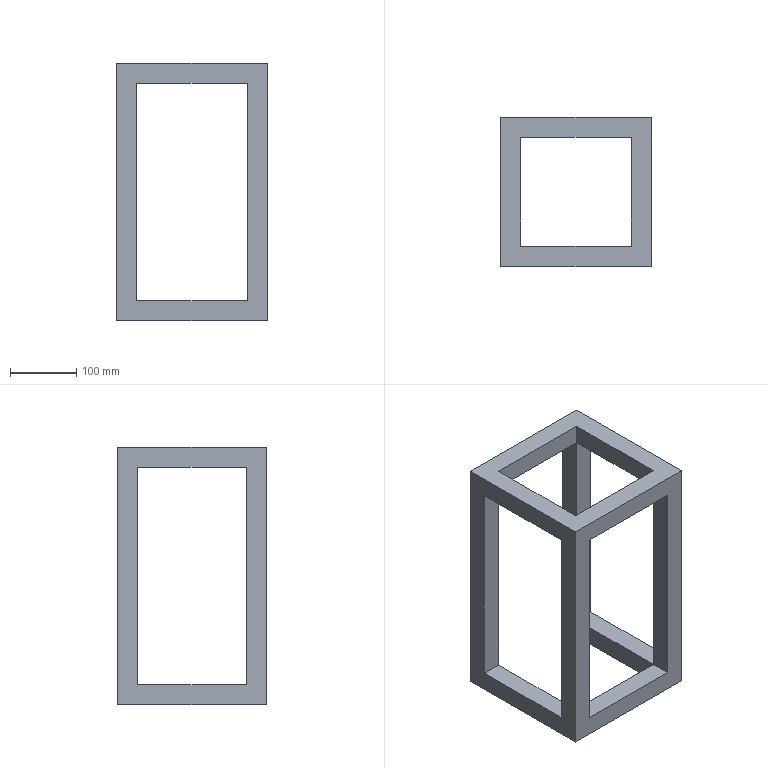Part | STEP file | 1 solid | 26 faces | box 226.259 x 224 x 387.57 mm | volume 2434549 mm3 | plane 26